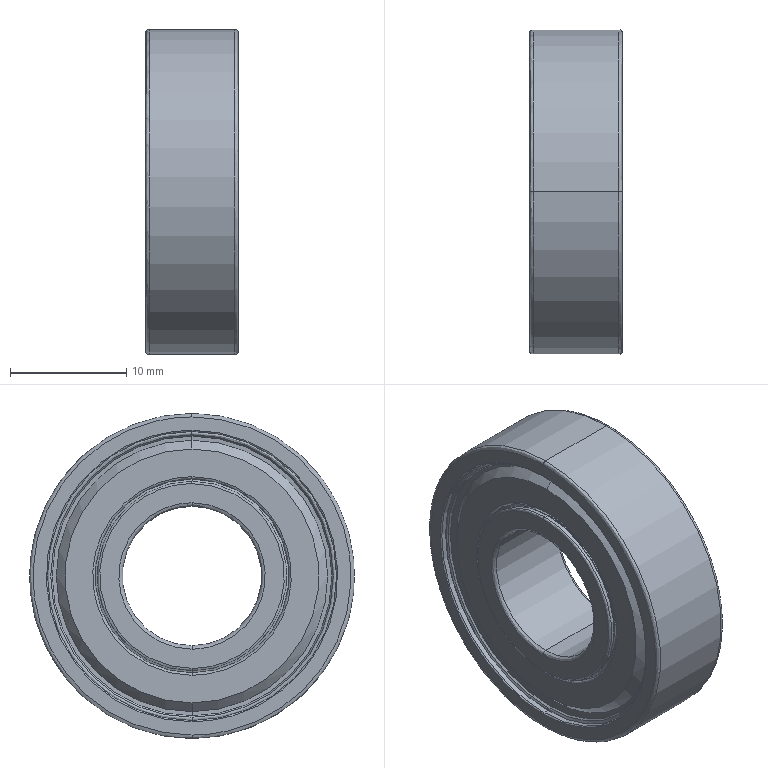Part | SolidWorks | features BaseBody 1 | 1 solid | 136 faces | box 8 x 28 x 28 mm | volume 3202 mm3 | spline 52 | cone 40 | cylinder 32 | plane 12 | commonest cylinder face diameters 15.5 x4 16.3 x4 16.7 x4 17.1 x4 17.5 x4 23.5 x4